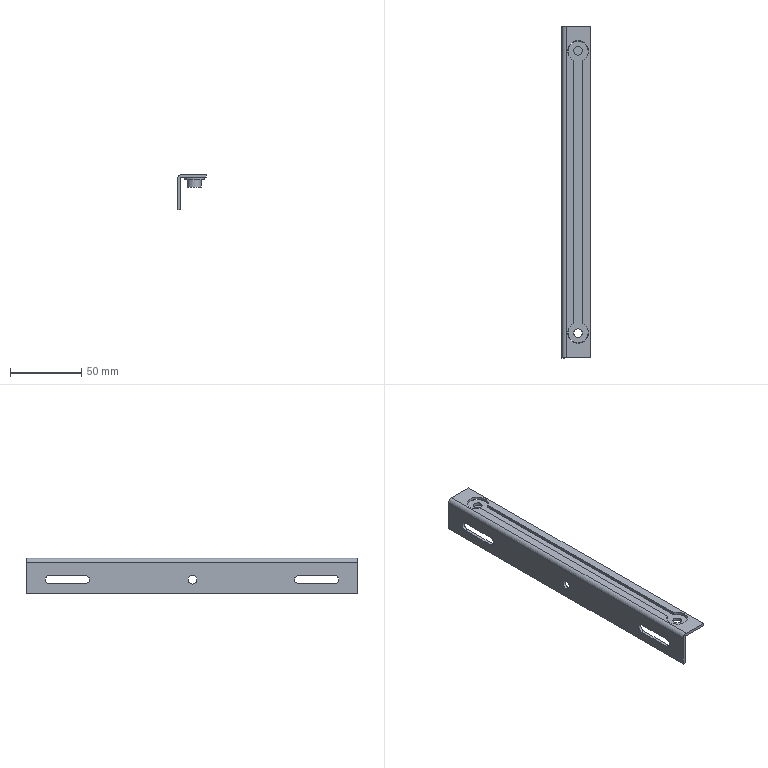Part | SolidWorks | features ICE 4, Extrusion 1 | 2 solids | 42 faces | box 20 x 233 x 25 mm | volume 22029 mm3 | cylinder 22 | plane 20 | commonest cylinder face diameters 14.5 x6 6 x5 6.2 x4 6.3 x2 9.952 x2 14 x2
STEP:
#1=CARTESIAN_POINT('',(-5.5,17.5,-4.));
#2=VERTEX_POINT('',#1);
#3=CARTESIAN_POINT('',(-11.5,17.5,-4.));
#4=VERTEX_POINT('',#3);
#5=CARTESIAN_POINT('',(-8.5,17.5,-4.));
#6=DIRECTION('',(0.,0.,-1.));
#7=DIRECTION('',(-1.,0.,0.));
#8=AXIS2_PLACEMENT_3D('',#5,#6,#7);
#9=CIRCLE('',#8,3.);
#10=EDGE_CURVE('',#2,#4,#9,.T.);
#11=ORIENTED_EDGE('',*,*,#10,.T.);
#12=CARTESIAN_POINT('',(-11.5,17.5,-2.));
#13=VERTEX_POINT('',#12);
#14=CARTESIAN_POINT('',(-11.5,17.5,-4.));
#15=DIRECTION('',(0.,0.,1.));
#16=VECTOR('',#15,1000.);
#17=LINE('',#14,#16);
#18=EDGE_CURVE('',#4,#13,#17,.T.);
#19=ORIENTED_EDGE('',*,*,#18,.T.);
#20=CARTESIAN_POINT('',(-5.5,17.5,-2.));
#21=VERTEX_POINT('',#20);
#22=CARTESIAN_POINT('',(-8.5,17.5,-2.));
#23=DIRECTION('',(0.,0.,-1.));
#24=DIRECTION('',(-1.,0.,0.));
#25=AXIS2_PLACEMENT_3D('',#22,#23,#24);
#26=CIRCLE('',#25,3.);
#27=EDGE_CURVE('',#21,#13,#26,.T.);
#28=ORIENTED_EDGE('',*,*,#27,.F.);
#29=CARTESIAN_POINT('',(-5.5,17.5,-4.));
#30=DIRECTION('',(0.,0.,1.));
#31=VECTOR('',#30,1000.);
#32=LINE('',#29,#31);
#33=EDGE_CURVE('',#2,#21,#32,.T.);
#34=ORIENTED_EDGE('',*,*,#33,.F.);
#35=EDGE_LOOP('',(#11,#19,#28,#34));
#36=FACE_OUTER_BOUND('',#35,.T.);
#37=CARTESIAN_POINT('',(-8.5,17.5,-4.));
#38=DIRECTION('',(0.,0.,1.));
#39=DIRECTION('',(1.,0.,0.));
#40=AXIS2_PLACEMENT_3D('',#37,#38,#39);
#41=CYLINDRICAL_SURFACE('',#40,3.);
#42=ADVANCED_FACE('',(#36),#41,.F.);
#43=CARTESIAN_POINT('',(-5.5,215.5,-4.));
#44=VERTEX_POINT('',#43);
#45=CARTESIAN_POINT('',(-11.5,215.5,-4.));
#46=VERTEX_POINT('',#45);
#47=CARTESIAN_POINT('',(-8.5,215.5,-4.));
#48=DIRECTION('',(0.,0.,-1.));
#49=DIRECTION('',(-1.,0.,0.));
#50=AXIS2_PLACEMENT_3D('',#47,#48,#49);
#51=CIRCLE('',#50,3.);
#52=EDGE_CURVE('',#44,#46,#51,.T.);
#53=ORIENTED_EDGE('',*,*,#52,.T.);
#54=CARTESIAN_POINT('',(-11.5,215.5,-2.));
#55=VERTEX_POINT('',#54);
#56=CARTESIAN_POINT('',(-11.5,215.5,-4.));
#57=DIRECTION('',(0.,0.,1.));
#58=VECTOR('',#57,1000.);
#59=LINE('',#56,#58);
#60=EDGE_CURVE('',#46,#55,#59,.T.);
#61=ORIENTED_EDGE('',*,*,#60,.T.);
#62=CARTESIAN_POINT('',(-5.5,215.5,-2.));
#63=VERTEX_POINT('',#62);
#64=CARTESIAN_POINT('',(-8.5,215.5,-2.));
#65=DIRECTION('',(0.,0.,-1.));
#66=DIRECTION('',(-1.,0.,0.));
#67=AXIS2_PLACEMENT_3D('',#64,#65,#66);
#68=CIRCLE('',#67,3.);
#69=EDGE_CURVE('',#63,#55,#68,.T.);
#70=ORIENTED_EDGE('',*,*,#69,.F.);
#71=CARTESIAN_POINT('',(-5.5,215.5,-4.));
#72=DIRECTION('',(0.,0.,1.));
#73=VECTOR('',#72,1000.);
#74=LINE('',#71,#73);
#75=EDGE_CURVE('',#44,#63,#74,.T.);
#76=ORIENTED_EDGE('',*,*,#75,.F.);
#77=EDGE_LOOP('',(#53,#61,#70,#76));
#78=FACE_OUTER_BOUND('',#77,.T.);
#79=CARTESIAN_POINT('',(-8.5,215.5,-4.));
#80=DIRECTION('',(0.,0.,1.));
#81=DIRECTION('',(1.,0.,0.));
#82=AXIS2_PLACEMENT_3D('',#79,#80,#81);
#83=CYLINDRICAL_SURFACE('',#82,3.);
#84=ADVANCED_FACE('',(#78),#83,.F.);
#85=CARTESIAN_POINT('',(-1.25,215.5,0.));
#86=VERTEX_POINT('',#85);
#87=CARTESIAN_POINT('',(-5.4,208.946,0.));
#88=VERTEX_POINT('',#87);
#89=CARTESIAN_POINT('',(-8.5,215.5,0.));
#90=DIRECTION('',(0.,0.,-1.));
#91=DIRECTION('',(-1.,0.,0.));
#92=AXIS2_PLACEMENT_3D('',#89,#90,#91);
#93=CIRCLE('',#92,7.25);
#94=EDGE_CURVE('',#86,#88,#93,.T.);
#95=ORIENTED_EDGE('',*,*,#94,.F.);
#96=CARTESIAN_POINT('',(-1.25,215.5,-2.));
#97=VERTEX_POINT('',#96);
#98=CARTESIAN_POINT('',(-1.25,215.5,0.));
#99=DIRECTION('',(0.,0.,-1.));
#100=VECTOR('',#99,1000.);
#101=LINE('',#98,#100);
#102=EDGE_CURVE('',#86,#97,#101,.T.);
#103=ORIENTED_EDGE('',*,*,#102,.T.);
#104=CARTESIAN_POINT('',(-1.5,213.613,-2.));
#105=VERTEX_POINT('',#104);
#106=CARTESIAN_POINT('',(-8.5,215.5,-2.));
#107=DIRECTION('',(0.,0.,-1.));
#108=DIRECTION('',(-1.,0.,0.));
#109=AXIS2_PLACEMENT_3D('',#106,#107,#108);
#110=CIRCLE('',#109,7.25);
#111=EDGE_CURVE('',#97,#105,#110,.T.);
#112=ORIENTED_EDGE('',*,*,#111,.T.);
#113=CARTESIAN_POINT('',(-5.4,208.946,-2.));
#114=VERTEX_POINT('',#113);
#115=CARTESIAN_POINT('',(-8.5,215.5,-2.));
#116=DIRECTION('',(0.,0.,1.));
#117=DIRECTION('',(-1.,0.,0.));
#118=AXIS2_PLACEMENT_3D('',#115,#116,#117);
#119=CIRCLE('',#118,7.25);
#120=EDGE_CURVE('',#114,#105,#119,.T.);
#121=ORIENTED_EDGE('',*,*,#120,.F.);
#122=CARTESIAN_POINT('',(-5.4,208.946,0.));
#123=DIRECTION('',(0.,0.,-1.));
#124=VECTOR('',#123,1000.);
#125=LINE('',#122,#124);
#126=EDGE_CURVE('',#88,#114,#125,.T.);
#127=ORIENTED_EDGE('',*,*,#126,.F.);
#128=EDGE_LOOP('',(#95,#103,#112,#121,#127));
#129=FACE_OUTER_BOUND('',#128,.T.);
#130=CARTESIAN_POINT('',(-8.5,215.5,0.));
#131=DIRECTION('',(0.,0.,-1.));
#132=DIRECTION('',(-1.,0.,0.));
#133=AXIS2_PLACEMENT_3D('',#130,#131,#132);
#134=CYLINDRICAL_SURFACE('',#133,7.25);
#135=ADVANCED_FACE('',(#129),#134,.F.);
#136=ORIENTED_EDGE('',*,*,#102,.F.);
#137=CARTESIAN_POINT('',(-15.75,215.5,0.));
#138=VERTEX_POINT('',#137);
#139=CARTESIAN_POINT('',(-8.5,215.5,0.));
#140=DIRECTION('',(0.,0.,-1.));
#141=DIRECTION('',(-1.,0.,0.));
#142=AXIS2_PLACEMENT_3D('',#139,#140,#141);
#143=CIRCLE('',#142,7.25);
#144=EDGE_CURVE('',#138,#86,#143,.T.);
#145=ORIENTED_EDGE('',*,*,#144,.F.);
#146=CARTESIAN_POINT('',(-15.75,215.5,-2.));
#147=VERTEX_POINT('',#146);
#148=CARTESIAN_POINT('',(-15.75,215.5,0.));
#149=DIRECTION('',(0.,0.,-1.));
#150=VECTOR('',#149,1000.);
#151=LINE('',#148,#150);
#152=EDGE_CURVE('',#138,#147,#151,.T.);
#153=ORIENTED_EDGE('',*,*,#152,.T.);
#154=CARTESIAN_POINT('',(-8.5,215.5,-2.));
#155=DIRECTION('',(0.,0.,-1.));
#156=DIRECTION('',(-1.,0.,0.));
#157=AXIS2_PLACEMENT_3D('',#154,#155,#156);
#158=CIRCLE('',#157,7.25);
#159=EDGE_CURVE('',#147,#97,#158,.T.);
#160=ORIENTED_EDGE('',*,*,#159,.T.);
#161=EDGE_LOOP('',(#136,#145,#153,#160));
#162=FACE_OUTER_BOUND('',#161,.T.);
#163=CARTESIAN_POINT('',(-8.5,215.5,0.));
#164=DIRECTION('',(0.,0.,-1.));
#165=DIRECTION('',(-1.,0.,0.));
#166=AXIS2_PLACEMENT_3D('',#163,#164,#165);
#167=CYLINDRICAL_SURFACE('',#166,7.25);
#168=ADVANCED_FACE('',(#162),#167,.F.);
#169=CARTESIAN_POINT('',(-1.25,17.5,0.));
#170=VERTEX_POINT('',#169);
#171=CARTESIAN_POINT('',(-15.75,17.5,0.));
#172=VERTEX_POINT('',#171);
#173=CARTESIAN_POINT('',(-8.5,17.5,0.));
#174=DIRECTION('',(0.,0.,-1.));
#175=DIRECTION('',(-1.,0.,0.));
#176=AXIS2_PLACEMENT_3D('',#173,#174,#175);
#177=CIRCLE('',#176,7.25);
#178=EDGE_CURVE('',#170,#172,#177,.T.);
#179=ORIENTED_EDGE('',*,*,#178,.F.);
#180=CARTESIAN_POINT('',(-1.25,17.5,-2.));
#181=VERTEX_POINT('',#180);
#182=CARTESIAN_POINT('',(-1.25,17.5,0.));
#183=DIRECTION('',(0.,0.,-1.));
#184=VECTOR('',#183,1000.);
#185=LINE('',#182,#184);
#186=EDGE_CURVE('',#170,#181,#185,.T.);
#187=ORIENTED_EDGE('',*,*,#186,.T.);
#188=CARTESIAN_POINT('',(-15.75,17.5,-2.));
#189=VERTEX_POINT('',#188);
#190=CARTESIAN_POINT('',(-8.5,17.5,-2.));
#191=DIRECTION('',(0.,0.,-1.));
#192=DIRECTION('',(-1.,0.,0.));
#193=AXIS2_PLACEMENT_3D('',#190,#191,#192);
#194=CIRCLE('',#193,7.25);
#195=EDGE_CURVE('',#181,#189,#194,.T.);
#196=ORIENTED_EDGE('',*,*,#195,.T.);
#197=CARTESIAN_POINT('',(-15.75,17.5,0.));
#198=DIRECTION('',(0.,0.,-1.));
#199=VECTOR('',#198,1000.);
#200=LINE('',#197,#199);
#201=EDGE_CURVE('',#172,#189,#200,.T.);
#202=ORIENTED_EDGE('',*,*,#201,.F.);
#203=EDGE_LOOP('',(#179,#187,#196,#202));
#204=FACE_OUTER_BOUND('',#203,.T.);
#205=CARTESIAN_POINT('',(-8.5,17.5,0.));
#206=DIRECTION('',(0.,0.,-1.));
#207=DIRECTION('',(-1.,0.,0.));
#208=AXIS2_PLACEMENT_3D('',#205,#206,#207);
#209=CYLINDRICAL_SURFACE('',#208,7.25);
#210=ADVANCED_FACE('',(#204),#209,.F.);
#211=CARTESIAN_POINT('',(-11.6,24.054,0.));
#212=VERTEX_POINT('',#211);
#213=CARTESIAN_POINT('',(-8.5,17.5,0.));
#214=DIRECTION('',(0.,0.,-1.));
#215=DIRECTION('',(-1.,0.,0.));
#216=AXIS2_PLACEMENT_3D('',#213,#214,#215);
#217=CIRCLE('',#216,7.25);
#218=EDGE_CURVE('',#172,#212,#217,.T.);
#219=ORIENTED_EDGE('',*,*,#218,.F.);
#220=ORIENTED_EDGE('',*,*,#201,.T.);
#221=CARTESIAN_POINT('',(-15.5,19.387,-2.));
#222=VERTEX_POINT('',#221);
#223=CARTESIAN_POINT('',(-8.5,17.5,-2.));
#224=DIRECTION('',(0.,0.,-1.));
#225=DIRECTION('',(-1.,0.,0.));
#226=AXIS2_PLACEMENT_3D('',#223,#224,#225);
#227=CIRCLE('',#226,7.25);
#228=EDGE_CURVE('',#189,#222,#227,.T.);
#229=ORIENTED_EDGE('',*,*,#228,.T.);
#230=CARTESIAN_POINT('',(-11.6,24.054,-2.));
#231=VERTEX_POINT('',#230);
#232=CARTESIAN_POINT('',(-8.5,17.5,-2.));
#233=DIRECTION('',(0.,0.,1.));
#234=DIRECTION('',(-1.,0.,0.));
#235=AXIS2_PLACEMENT_3D('',#232,#233,#234);
#236=CIRCLE('',#235,7.25);
#237=EDGE_CURVE('',#231,#222,#236,.T.);
#238=ORIENTED_EDGE('',*,*,#237,.F.);
#239=CARTESIAN_POINT('',(-11.6,24.054,0.));
#240=DIRECTION('',(0.,0.,-1.));
#241=VECTOR('',#240,1000.);
#242=LINE('',#239,#241);
#243=EDGE_CURVE('',#212,#231,#242,.T.);
#244=ORIENTED_EDGE('',*,*,#243,.F.);
#245=EDGE_LOOP('',(#219,#220,#229,#238,#244));
#246=FACE_OUTER_BOUND('',#245,.T.);
#247=CARTESIAN_POINT('',(-8.5,17.5,0.));
#248=DIRECTION('',(0.,0.,-1.));
#249=DIRECTION('',(-1.,0.,0.));
#250=AXIS2_PLACEMENT_3D('',#247,#248,#249);
#251=CYLINDRICAL_SURFACE('',#250,7.25);
#252=ADVANCED_FACE('',(#246),#251,.F.);
#253=CARTESIAN_POINT('',(-20.,116.173,-11.85));
#254=VERTEX_POINT('',#253);
#255=CARTESIAN_POINT('',(-20.,116.173,-18.15));
#256=VERTEX_POINT('',#255);
#257=CARTESIAN_POINT('',(-20.,116.173,-15.));
#258=DIRECTION('',(1.,0.,0.));
#259=DIRECTION('',(0.,0.,-1.));
#260=AXIS2_PLACEMENT_3D('',#257,#258,#259);
#261=CIRCLE('',#260,3.15);
#262=EDGE_CURVE('',#254,#256,#261,.T.);
#263=ORIENTED_EDGE('',*,*,#262,.F.);
#264=CARTESIAN_POINT('',(-18.,116.173,-11.85));
#265=VERTEX_POINT('',#264);
#266=CARTESIAN_POINT('',(-20.,116.173,-11.85));
#267=DIRECTION('',(1.,0.,0.));
#268=VECTOR('',#267,1000.);
#269=LINE('',#266,#268);
#270=EDGE_CURVE('',#254,#265,#269,.T.);
#271=ORIENTED_EDGE('',*,*,#270,.T.);
#272=CARTESIAN_POINT('',(-18.,116.173,-18.15));
#273=VERTEX_POINT('',#272);
#274=CARTESIAN_POINT('',(-18.,116.173,-15.));
#275=DIRECTION('',(-1.,0.,0.));
#276=DIRECTION('',(0.,0.,1.));
#277=AXIS2_PLACEMENT_3D('',#274,#275,#276);
#278=CIRCLE('',#277,3.15);
#279=EDGE_CURVE('',#273,#265,#278,.T.);
#280=ORIENTED_EDGE('',*,*,#279,.F.);
#281=CARTESIAN_POINT('',(-20.,116.173,-18.15));
#282=DIRECTION('',(1.,0.,0.));
#283=VECTOR('',#282,1000.);
#284=LINE('',#281,#283);
#285=EDGE_CURVE('',#256,#273,#284,.T.);
#286=ORIENTED_EDGE('',*,*,#285,.F.);
#287=EDGE_LOOP('',(#263,#271,#280,#286));
#288=FACE_OUTER_BOUND('',#287,.T.);
#289=CARTESIAN_POINT('',(-20.,116.173,-15.));
#290=DIRECTION('',(1.,0.,0.));
#291=DIRECTION('',(0.,0.,-1.));
#292=AXIS2_PLACEMENT_3D('',#289,#290,#291);
#293=CYLINDRICAL_SURFACE('',#292,3.15);
#294=ADVANCED_FACE('',(#288),#293,.F.);
#295=CARTESIAN_POINT('',(0.,0.,-2.));
#296=VERTEX_POINT('',#295);
#297=CARTESIAN_POINT('',(-17.,0.,-2.));
#298=VERTEX_POINT('',#297);
#299=CARTESIAN_POINT('',(0.,0.,-2.));
#300=DIRECTION('',(-1.,0.,0.));
#301=VECTOR('',#300,1000.);
#302=LINE('',#299,#301);
#303=EDGE_CURVE('',#296,#298,#302,.T.);
#304=ORIENTED_EDGE('',*,*,#303,.T.);
#305=CARTESIAN_POINT('',(-17.,233.,-2.));
#306=VERTEX_POINT('',#305);
#307=CARTESIAN_POINT('',(-17.,233.,-2.));
#308=DIRECTION('',(0.,-1.,0.));
#309=VECTOR('',#308,1000.);
#310=LINE('',#307,#309);
#311=EDGE_CURVE('',#306,#298,#310,.T.);
#312=ORIENTED_EDGE('',*,*,#311,.F.);
#313=CARTESIAN_POINT('',(0.,233.,-2.));
#314=VERTEX_POINT('',#313);
#315=CARTESIAN_POINT('',(0.,233.,-2.));
#316=DIRECTION('',(-1.,0.,0.));
#317=VECTOR('',#316,1000.);
#318=LINE('',#315,#317);
#319=EDGE_CURVE('',#314,#306,#318,.T.);
#320=ORIENTED_EDGE('',*,*,#319,.F.);
#321=CARTESIAN_POINT('',(0.,233.,-2.));
#322=DIRECTION('',(0.,-1.,0.));
#323=VECTOR('',#322,1000.);
#324=LINE('',#321,#323);
#325=EDGE_CURVE('',#314,#296,#324,.T.);
#326=ORIENTED_EDGE('',*,*,#325,.T.);
#327=EDGE_LOOP('',(#304,#312,#320,#326));
#328=FACE_OUTER_BOUND('',#327,.T.);
#329=CARTESIAN_POINT('',(-15.5,213.613,-2.));
#330=VERTEX_POINT('',#329);
#331=CARTESIAN_POINT('',(-15.5,215.5,-2.));
#332=DIRECTION('',(0.,1.,0.));
#333=VECTOR('',#332,1000.);
#334=LINE('',#331,#333);
#335=EDGE_CURVE('',#222,#330,#334,.T.);
#336=ORIENTED_EDGE('',*,*,#335,.F.);
#337=ORIENTED_EDGE('',*,*,#228,.F.);
#338=ORIENTED_EDGE('',*,*,#195,.F.);
#339=CARTESIAN_POINT('',(-1.5,19.387,-2.));
#340=VERTEX_POINT('',#339);
#341=CARTESIAN_POINT('',(-8.5,17.5,-2.));
#342=DIRECTION('',(0.,0.,-1.));
#343=DIRECTION('',(-1.,0.,0.));
#344=AXIS2_PLACEMENT_3D('',#341,#342,#343);
#345=CIRCLE('',#344,7.25);
#346=EDGE_CURVE('',#340,#181,#345,.T.);
#347=ORIENTED_EDGE('',*,*,#346,.F.);
#348=CARTESIAN_POINT('',(-1.5,215.5,-2.));
#349=DIRECTION('',(0.,-1.,0.));
#350=VECTOR('',#349,1000.);
#351=LINE('',#348,#350);
#352=EDGE_CURVE('',#105,#340,#351,.T.);
#353=ORIENTED_EDGE('',*,*,#352,.F.);
#354=ORIENTED_EDGE('',*,*,#111,.F.);
#355=ORIENTED_EDGE('',*,*,#159,.F.);
#356=CARTESIAN_POINT('',(-8.5,215.5,-2.));
#357=DIRECTION('',(0.,0.,-1.));
#358=DIRECTION('',(-1.,0.,0.));
#359=AXIS2_PLACEMENT_3D('',#356,#357,#358);
#360=CIRCLE('',#359,7.25);
#361=EDGE_CURVE('',#330,#147,#360,.T.);
#362=ORIENTED_EDGE('',*,*,#361,.F.);
#363=EDGE_LOOP('',(#336,#337,#338,#347,#353,#354,#355,#362));
#364=FACE_BOUND('',#363,.T.);
#365=CARTESIAN_POINT('',(0.,233.,-2.));
#366=DIRECTION('',(0.,0.,1.));
#367=DIRECTION('',(1.,0.,0.));
#368=AXIS2_PLACEMENT_3D('',#365,#366,#367);
#369=PLANE('',#368);
#370=ADVANCED_FACE('',(#328,#364),#369,.F.);
#371=CARTESIAN_POINT('',(0.,0.,0.));
#372=VERTEX_POINT('',#371);
#373=CARTESIAN_POINT('',(0.,0.,-2.));
#374=DIRECTION('',(0.,0.,-1.));
#375=VECTOR('',#374,1000.);
#376=LINE('',#373,#375);
#377=EDGE_CURVE('',#372,#296,#376,.T.);
#378=ORIENTED_EDGE('',*,*,#377,.T.);
#379=ORIENTED_EDGE('',*,*,#325,.F.);
#380=CARTESIAN_POINT('',(0.,233.,0.));
#381=VERTEX_POINT('',#380);
#382=CARTESIAN_POINT('',(0.,233.,-2.));
#383=DIRECTION('',(0.,0.,-1.));
#384=VECTOR('',#383,1000.);
#385=LINE('',#382,#384);
#386=EDGE_CURVE('',#381,#314,#385,.T.);
#387=ORIENTED_EDGE('',*,*,#386,.F.);
#388=CARTESIAN_POINT('',(0.,233.,0.));
#389=DIRECTION('',(0.,-1.,0.));
#390=VECTOR('',#389,1000.);
#391=LINE('',#388,#390);
#392=EDGE_CURVE('',#381,#372,#391,.T.);
#393=ORIENTED_EDGE('',*,*,#392,.T.);
#394=EDGE_LOOP('',(#378,#379,#387,#393));
#395=FACE_OUTER_BOUND('',#394,.T.);
#396=CARTESIAN_POINT('',(0.,233.,-2.));
#397=DIRECTION('',(-1.,0.,0.));
#398=DIRECTION('',(0.,0.,1.));
#399=AXIS2_PLACEMENT_3D('',#396,#397,#398);
#400=PLANE('',#399);
#401=ADVANCED_FACE('',(#395),#400,.F.);
#402=CARTESIAN_POINT('',(-18.,0.,-3.));
#403=VERTEX_POINT('',#402);
#404=CARTESIAN_POINT('',(-17.,0.,-3.));
#405=DIRECTION('',(0.,-1.,0.));
#406=DIRECTION('',(0.,0.,-1.));
#407=AXIS2_PLACEMENT_3D('',#404,#405,#406);
#408=CIRCLE('',#407,1.);
#409=EDGE_CURVE('',#298,#403,#408,.T.);
#410=ORIENTED_EDGE('',*,*,#409,.T.);
#411=CARTESIAN_POINT('',(-18.,233.,-3.));
#412=VERTEX_POINT('',#411);
#413=CARTESIAN_POINT('',(-18.,233.,-3.));
#414=DIRECTION('',(0.,-1.,0.));
#415=VECTOR('',#414,1000.);
#416=LINE('',#413,#415);
#417=EDGE_CURVE('',#412,#403,#416,.T.);
#418=ORIENTED_EDGE('',*,*,#417,.F.);
#419=CARTESIAN_POINT('',(-17.,233.,-3.));
#420=DIRECTION('',(0.,-1.,0.));
#421=DIRECTION('',(0.,0.,-1.));
#422=AXIS2_PLACEMENT_3D('',#419,#420,#421);
#423=CIRCLE('',#422,1.);
#424=EDGE_CURVE('',#306,#412,#423,.T.);
#425=ORIENTED_EDGE('',*,*,#424,.F.);
#426=ORIENTED_EDGE('',*,*,#311,.T.);
#427=EDGE_LOOP('',(#410,#418,#425,#426));
#428=FACE_OUTER_BOUND('',#427,.T.);
#429=CARTESIAN_POINT('',(-17.,233.,-3.));
#430=DIRECTION('',(0.,-1.,0.));
#431=DIRECTION('',(0.,0.,-1.));
#432=AXIS2_PLACEMENT_3D('',#429,#430,#431);
#433=CYLINDRICAL_SURFACE('',#432,1.);
#434=ADVANCED_FACE('',(#428),#433,.F.);
#435=CARTESIAN_POINT('',(-18.,191.65,-11.9));
#436=VERTEX_POINT('',#435);
#437=CARTESIAN_POINT('',(-18.,216.35,-11.9));
#438=VERTEX_POINT('',#437);
#439=CARTESIAN_POINT('',(-18.,233.,-11.9));
#440=DIRECTION('',(0.,1.,0.));
#441=VECTOR('',#440,1000.);
#442=LINE('',#439,#441);
#443=EDGE_CURVE('',#436,#438,#442,.T.);
#444=ORIENTED_EDGE('',*,*,#443,.T.);
#445=CARTESIAN_POINT('',(-18.,216.35,-18.1));
#446=VERTEX_POINT('',#445);
#447=CARTESIAN_POINT('',(-18.,216.35,-15.));
#448=DIRECTION('',(-1.,0.,0.));
#449=DIRECTION('',(0.,0.,1.));
#450=AXIS2_PLACEMENT_3D('',#447,#448,#449);
#451=CIRCLE('',#450,3.1);
#452=EDGE_CURVE('',#438,#446,#451,.T.);
#453=ORIENTED_EDGE('',*,*,#452,.T.);
#454=CARTESIAN_POINT('',(-18.,191.65,-18.1));
#455=VERTEX_POINT('',#454);
#456=CARTESIAN_POINT('',(-18.,233.,-18.1));
#457=DIRECTION('',(0.,-1.,0.));
#458=VECTOR('',#457,1000.);
#459=LINE('',#456,#458);
#460=EDGE_CURVE('',#446,#455,#459,.T.);
#461=ORIENTED_EDGE('',*,*,#460,.T.);
#462=CARTESIAN_POINT('',(-18.,191.65,-15.));
#463=DIRECTION('',(-1.,0.,0.));
#464=DIRECTION('',(0.,0.,1.));
#465=AXIS2_PLACEMENT_3D('',#462,#463,#464);
#466=CIRCLE('',#465,3.1);
#467=EDGE_CURVE('',#455,#436,#466,.T.);
#468=ORIENTED_EDGE('',*,*,#467,.T.);
#469=EDGE_LOOP('',(#444,#453,#461,#468));
#470=FACE_BOUND('',#469,.T.);
#471=CARTESIAN_POINT('',(-18.,16.65,-11.9));
#472=VERTEX_POINT('',#471);
#473=CARTESIAN_POINT('',(-18.,41.35,-11.9));
#474=VERTEX_POINT('',#473);
#475=CARTESIAN_POINT('',(-18.,233.,-11.9));
#476=DIRECTION('',(0.,1.,0.));
#477=VECTOR('',#476,1000.);
#478=LINE('',#475,#477);
#479=EDGE_CURVE('',#472,#474,#478,.T.);
#480=ORIENTED_EDGE('',*,*,#479,.T.);
#481=CARTESIAN_POINT('',(-18.,41.35,-18.1));
#482=VERTEX_POINT('',#481);
#483=CARTESIAN_POINT('',(-18.,41.35,-15.));
#484=DIRECTION('',(-1.,0.,0.));
#485=DIRECTION('',(0.,0.,1.));
#486=AXIS2_PLACEMENT_3D('',#483,#484,#485);
#487=CIRCLE('',#486,3.1);
#488=EDGE_CURVE('',#474,#482,#487,.T.);
#489=ORIENTED_EDGE('',*,*,#488,.T.);
#490=CARTESIAN_POINT('',(-18.,16.65,-18.1));
#491=VERTEX_POINT('',#490);
#492=CARTESIAN_POINT('',(-18.,233.,-18.1));
#493=DIRECTION('',(0.,-1.,0.));
#494=VECTOR('',#493,1000.);
#495=LINE('',#492,#494);
#496=EDGE_CURVE('',#482,#491,#495,.T.);
#497=ORIENTED_EDGE('',*,*,#496,.T.);
#498=CARTESIAN_POINT('',(-18.,16.65,-15.));
#499=DIRECTION('',(-1.,0.,0.));
#500=DIRECTION('',(0.,0.,1.));
#501=AXIS2_PLACEMENT_3D('',#498,#499,#500);
#502=CIRCLE('',#501,3.1);
#503=EDGE_CURVE('',#491,#472,#502,.T.);
#504=ORIENTED_EDGE('',*,*,#503,.T.);
#505=EDGE_LOOP('',(#480,#489,#497,#504));
#506=FACE_BOUND('',#505,.T.);
#507=ORIENTED_EDGE('',*,*,#279,.T.);
#508=CARTESIAN_POINT('',(-18.,116.173,-15.));
#509=DIRECTION('',(-1.,0.,0.));
#510=DIRECTION('',(0.,0.,1.));
#511=AXIS2_PLACEMENT_3D('',#508,#509,#510);
#512=CIRCLE('',#511,3.15);
#513=EDGE_CURVE('',#265,#273,#512,.T.);
#514=ORIENTED_EDGE('',*,*,#513,.T.);
#515=EDGE_LOOP('',(#507,#514));
#516=FACE_BOUND('',#515,.T.);
#517=CARTESIAN_POINT('',(-18.,0.,-25.));
#518=VERTEX_POINT('',#517);
#519=CARTESIAN_POINT('',(-18.,0.,-25.));
#520=DIRECTION('',(0.,0.,-1.));
#521=VECTOR('',#520,1000.);
#522=LINE('',#519,#521);
#523=EDGE_CURVE('',#403,#518,#522,.T.);
#524=ORIENTED_EDGE('',*,*,#523,.T.);
#525=CARTESIAN_POINT('',(-18.,233.,-25.));
#526=VERTEX_POINT('',#525);
#527=CARTESIAN_POINT('',(-18.,233.,-25.));
#528=DIRECTION('',(0.,-1.,0.));
#529=VECTOR('',#528,1000.);
#530=LINE('',#527,#529);
#531=EDGE_CURVE('',#526,#518,#530,.T.);
#532=ORIENTED_EDGE('',*,*,#531,.F.);
#533=CARTESIAN_POINT('',(-18.,233.,-3.));
#534=DIRECTION('',(0.,0.,-1.));
#535=VECTOR('',#534,1000.);
#536=LINE('',#533,#535);
#537=EDGE_CURVE('',#412,#526,#536,.T.);
#538=ORIENTED_EDGE('',*,*,#537,.F.);
#539=ORIENTED_EDGE('',*,*,#417,.T.);
#540=EDGE_LOOP('',(#524,#532,#538,#539));
#541=FACE_OUTER_BOUND('',#540,.T.);
#542=CARTESIAN_POINT('',(-18.,233.,-25.));
#543=DIRECTION('',(-1.,0.,0.));
#544=DIRECTION('',(0.,0.,1.));
#545=AXIS2_PLACEMENT_3D('',#542,#543,#544);
#546=PLANE('',#545);
#547=ADVANCED_FACE('',(#470,#506,#516,#541),#546,.F.);
#548=CARTESIAN_POINT('',(-20.,0.,-25.));
#549=VERTEX_POINT('',#548);
#550=CARTESIAN_POINT('',(-20.,0.,-25.));
#551=DIRECTION('',(-1.,0.,0.));
#552=VECTOR('',#551,1000.);
#553=LINE('',#550,#552);
#554=EDGE_CURVE('',#518,#549,#553,.T.);
#555=ORIENTED_EDGE('',*,*,#554,.T.);
#556=CARTESIAN_POINT('',(-20.,233.,-25.));
#557=VERTEX_POINT('',#556);
#558=CARTESIAN_POINT('',(-20.,233.,-25.));
#559=DIRECTION('',(0.,-1.,0.));
#560=VECTOR('',#559,1000.);
#561=LINE('',#558,#560);
#562=EDGE_CURVE('',#557,#549,#561,.T.);
#563=ORIENTED_EDGE('',*,*,#562,.F.);
#564=CARTESIAN_POINT('',(-20.,233.,-25.));
#565=DIRECTION('',(-1.,0.,0.));
#566=VECTOR('',#565,1000.);
#567=LINE('',#564,#566);
#568=EDGE_CURVE('',#526,#557,#567,.T.);
#569=ORIENTED_EDGE('',*,*,#568,.F.);
#570=ORIENTED_EDGE('',*,*,#531,.T.);
#571=EDGE_LOOP('',(#555,#563,#569,#570));
#572=FACE_OUTER_BOUND('',#571,.T.);
#573=CARTESIAN_POINT('',(-20.,233.,-25.));
#574=DIRECTION('',(0.,0.,1.));
#575=DIRECTION('',(1.,0.,0.));
#576=AXIS2_PLACEMENT_3D('',#573,#574,#575);
#577=PLANE('',#576);
#578=ADVANCED_FACE('',(#572),#577,.F.);
#579=CARTESIAN_POINT('',(-20.,191.65,-18.1));
#580=VERTEX_POINT('',#579);
#581=CARTESIAN_POINT('',(-20.,216.35,-18.1));
#582=VERTEX_POINT('',#581);
#583=CARTESIAN_POINT('',(-20.,216.35,-18.1));
#584=DIRECTION('',(0.,1.,0.));
#585=VECTOR('',#584,1000.);
#586=LINE('',#583,#585);
#587=EDGE_CURVE('',#580,#582,#586,.T.);
#588=ORIENTED_EDGE('',*,*,#587,.T.);
#589=CARTESIAN_POINT('',(-20.,216.35,-11.9));
#590=VERTEX_POINT('',#589);
#591=CARTESIAN_POINT('',(-20.,216.35,-15.));
#592=DIRECTION('',(1.,0.,0.));
#593=DIRECTION('',(0.,0.,-1.));
#594=AXIS2_PLACEMENT_3D('',#591,#592,#593);
#595=CIRCLE('',#594,3.1);
#596=EDGE_CURVE('',#582,#590,#595,.T.);
#597=ORIENTED_EDGE('',*,*,#596,.T.);
#598=CARTESIAN_POINT('',(-20.,191.65,-11.9));
#599=VERTEX_POINT('',#598);
#600=CARTESIAN_POINT('',(-20.,216.35,-11.9));
#601=DIRECTION('',(0.,-1.,0.));
#602=VECTOR('',#601,1000.);
#603=LINE('',#600,#602);
#604=EDGE_CURVE('',#590,#599,#603,.T.);
#605=ORIENTED_EDGE('',*,*,#604,.T.);
#606=CARTESIAN_POINT('',(-20.,191.65,-15.));
#607=DIRECTION('',(1.,0.,0.));
#608=DIRECTION('',(0.,0.,-1.));
#609=AXIS2_PLACEMENT_3D('',#606,#607,#608);
#610=CIRCLE('',#609,3.1);
#611=EDGE_CURVE('',#599,#580,#610,.T.);
#612=ORIENTED_EDGE('',*,*,#611,.T.);
#613=EDGE_LOOP('',(#588,#597,#605,#612));
#614=FACE_BOUND('',#613,.T.);
#615=CARTESIAN_POINT('',(-20.,16.65,-18.1));
#616=VERTEX_POINT('',#615);
#617=CARTESIAN_POINT('',(-20.,41.35,-18.1));
#618=VERTEX_POINT('',#617);
#619=CARTESIAN_POINT('',(-20.,41.35,-18.1));
#620=DIRECTION('',(0.,1.,0.));
#621=VECTOR('',#620,1000.);
#622=LINE('',#619,#621);
#623=EDGE_CURVE('',#616,#618,#622,.T.);
#624=ORIENTED_EDGE('',*,*,#623,.T.);
#625=CARTESIAN_POINT('',(-20.,41.35,-11.9));
#626=VERTEX_POINT('',#625);
#627=CARTESIAN_POINT('',(-20.,41.35,-15.));
#628=DIRECTION('',(1.,0.,0.));
#629=DIRECTION('',(0.,0.,-1.));
#630=AXIS2_PLACEMENT_3D('',#627,#628,#629);
#631=CIRCLE('',#630,3.1);
#632=EDGE_CURVE('',#618,#626,#631,.T.);
#633=ORIENTED_EDGE('',*,*,#632,.T.);
#634=CARTESIAN_POINT('',(-20.,16.65,-11.9));
#635=VERTEX_POINT('',#634);
#636=CARTESIAN_POINT('',(-20.,41.35,-11.9));
#637=DIRECTION('',(0.,-1.,0.));
#638=VECTOR('',#637,1000.);
#639=LINE('',#636,#638);
#640=EDGE_CURVE('',#626,#635,#639,.T.);
#641=ORIENTED_EDGE('',*,*,#640,.T.);
#642=CARTESIAN_POINT('',(-20.,16.65,-15.));
#643=DIRECTION('',(1.,0.,0.));
#644=DIRECTION('',(0.,0.,-1.));
#645=AXIS2_PLACEMENT_3D('',#642,#643,#644);
#646=CIRCLE('',#645,3.1);
#647=EDGE_CURVE('',#635,#616,#646,.T.);
#648=ORIENTED_EDGE('',*,*,#647,.T.);
#649=EDGE_LOOP('',(#624,#633,#641,#648));
#650=FACE_BOUND('',#649,.T.);
#651=CARTESIAN_POINT('',(-20.,116.173,-15.));
#652=DIRECTION('',(1.,0.,0.));
#653=DIRECTION('',(0.,0.,-1.));
#654=AXIS2_PLACEMENT_3D('',#651,#652,#653);
#655=CIRCLE('',#654,3.15);
#656=EDGE_CURVE('',#256,#254,#655,.T.);
#657=ORIENTED_EDGE('',*,*,#656,.T.);
#658=ORIENTED_EDGE('',*,*,#262,.T.);
#659=EDGE_LOOP('',(#657,#658));
#660=FACE_BOUND('',#659,.T.);
#661=CARTESIAN_POINT('',(-20.,0.,-3.));
#662=VERTEX_POINT('',#661);
#663=CARTESIAN_POINT('',(-20.,0.,-3.));
#664=DIRECTION('',(0.,0.,1.));
#665=VECTOR('',#664,1000.);
#666=LINE('',#663,#665);
#667=EDGE_CURVE('',#549,#662,#666,.T.);
#668=ORIENTED_EDGE('',*,*,#667,.T.);
#669=CARTESIAN_POINT('',(-20.,233.,-3.));
#670=VERTEX_POINT('',#669);
#671=CARTESIAN_POINT('',(-20.,233.,-3.));
#672=DIRECTION('',(0.,-1.,0.));
#673=VECTOR('',#672,1000.);
#674=LINE('',#671,#673);
#675=EDGE_CURVE('',#670,#662,#674,.T.);
#676=ORIENTED_EDGE('',*,*,#675,.F.);
#677=CARTESIAN_POINT('',(-20.,233.,-8.424));
#678=DIRECTION('',(0.,0.,1.));
#679=VECTOR('',#678,1000.);
#680=LINE('',#677,#679);
#681=EDGE_CURVE('',#557,#670,#680,.T.);
#682=ORIENTED_EDGE('',*,*,#681,.F.);
#683=ORIENTED_EDGE('',*,*,#562,.T.);
#684=EDGE_LOOP('',(#668,#676,#682,#683));
#685=FACE_OUTER_BOUND('',#684,.T.);
#686=CARTESIAN_POINT('',(-20.,233.,-3.));
#687=DIRECTION('',(1.,0.,0.));
#688=DIRECTION('',(0.,0.,-1.));
#689=AXIS2_PLACEMENT_3D('',#686,#687,#688);
#690=PLANE('',#689);
#691=ADVANCED_FACE('',(#614,#650,#660,#685),#690,.F.);
#692=CARTESIAN_POINT('',(-17.,0.,0.));
#693=VERTEX_POINT('',#692);
#694=CARTESIAN_POINT('',(-17.,0.,-3.));
#695=DIRECTION('',(0.,1.,0.));
#696=DIRECTION('',(0.,0.,-1.));
#697=AXIS2_PLACEMENT_3D('',#694,#695,#696);
#698=CIRCLE('',#697,3.);
#699=EDGE_CURVE('',#662,#693,#698,.T.);
#700=ORIENTED_EDGE('',*,*,#699,.T.);
#701=CARTESIAN_POINT('',(-17.,233.,0.));
#702=VERTEX_POINT('',#701);
#703=CARTESIAN_POINT('',(-17.,233.,0.));
#704=DIRECTION('',(0.,-1.,0.));
#705=VECTOR('',#704,1000.);
#706=LINE('',#703,#705);
#707=EDGE_CURVE('',#702,#693,#706,.T.);
#708=ORIENTED_EDGE('',*,*,#707,.F.);
#709=CARTESIAN_POINT('',(-17.,233.,-3.));
#710=DIRECTION('',(0.,1.,0.));
#711=DIRECTION('',(0.,0.,-1.));
#712=AXIS2_PLACEMENT_3D('',#709,#710,#711);
#713=CIRCLE('',#712,3.);
#714=EDGE_CURVE('',#670,#702,#713,.T.);
#715=ORIENTED_EDGE('',*,*,#714,.F.);
#716=ORIENTED_EDGE('',*,*,#675,.T.);
#717=EDGE_LOOP('',(#700,#708,#715,#716));
#718=FACE_OUTER_BOUND('',#717,.T.);
#719=CARTESIAN_POINT('',(-17.,233.,-3.));
#720=DIRECTION('',(0.,-1.,0.));
#721=DIRECTION('',(0.,0.,-1.));
#722=AXIS2_PLACEMENT_3D('',#719,#720,#721);
#723=CYLINDRICAL_SURFACE('',#722,3.);
#724=ADVANCED_FACE('',(#718),#723,.T.);
#725=CARTESIAN_POINT('',(-5.4,24.054,0.));
#726=VERTEX_POINT('',#725);
#727=CARTESIAN_POINT('',(-5.4,208.946,0.));
#728=DIRECTION('',(0.,-1.,0.));
#729=VECTOR('',#728,1000.);
#730=LINE('',#727,#729);
#731=EDGE_CURVE('',#88,#726,#730,.T.);
#732=ORIENTED_EDGE('',*,*,#731,.T.);
#733=CARTESIAN_POINT('',(-8.5,17.5,0.));
#734=DIRECTION('',(0.,0.,-1.));
#735=DIRECTION('',(-1.,0.,0.));
#736=AXIS2_PLACEMENT_3D('',#733,#734,#735);
#737=CIRCLE('',#736,7.25);
#738=EDGE_CURVE('',#726,#170,#737,.T.);
#739=ORIENTED_EDGE('',*,*,#738,.T.);
#740=ORIENTED_EDGE('',*,*,#178,.T.);
#741=ORIENTED_EDGE('',*,*,#218,.T.);
#742=CARTESIAN_POINT('',(-11.6,208.946,0.));
#743=VERTEX_POINT('',#742);
#744=CARTESIAN_POINT('',(-11.6,208.946,0.));
#745=DIRECTION('',(0.,1.,0.));
#746=VECTOR('',#745,1000.);
#747=LINE('',#744,#746);
#748=EDGE_CURVE('',#212,#743,#747,.T.);
#749=ORIENTED_EDGE('',*,*,#748,.T.);
#750=CARTESIAN_POINT('',(-8.5,215.5,0.));
#751=DIRECTION('',(0.,0.,-1.));
#752=DIRECTION('',(-1.,0.,0.));
#753=AXIS2_PLACEMENT_3D('',#750,#751,#752);
#754=CIRCLE('',#753,7.25);
#755=EDGE_CURVE('',#743,#138,#754,.T.);
#756=ORIENTED_EDGE('',*,*,#755,.T.);
#757=ORIENTED_EDGE('',*,*,#144,.T.);
#758=ORIENTED_EDGE('',*,*,#94,.T.);
#759=EDGE_LOOP('',(#732,#739,#740,#741,#749,#756,#757,#758));
#760=FACE_BOUND('',#759,.T.);
#761=CARTESIAN_POINT('',(0.,0.,0.));
#762=DIRECTION('',(1.,0.,0.));
#763=VECTOR('',#762,1000.);
#764=LINE('',#761,#763);
#765=EDGE_CURVE('',#693,#372,#764,.T.);
#766=ORIENTED_EDGE('',*,*,#765,.T.);
#767=ORIENTED_EDGE('',*,*,#392,.F.);
#768=CARTESIAN_POINT('',(0.,233.,0.));
#769=DIRECTION('',(1.,0.,0.));
#770=VECTOR('',#769,1000.);
#771=LINE('',#768,#770);
#772=EDGE_CURVE('',#702,#381,#771,.T.);
#773=ORIENTED_EDGE('',*,*,#772,.F.);
#774=ORIENTED_EDGE('',*,*,#707,.T.);
#775=EDGE_LOOP('',(#766,#767,#773,#774));
#776=FACE_OUTER_BOUND('',#775,.T.);
#777=CARTESIAN_POINT('',(0.,233.,0.));
#778=DIRECTION('',(0.,0.,-1.));
#779=DIRECTION('',(-1.,0.,0.));
#780=AXIS2_PLACEMENT_3D('',#777,#778,#779);
#781=PLANE('',#780);
#782=ADVANCED_FACE('',(#760,#776),#781,.F.);
#783=ORIENTED_EDGE('',*,*,#386,.T.);
#784=ORIENTED_EDGE('',*,*,#319,.T.);
#785=ORIENTED_EDGE('',*,*,#424,.T.);
#786=ORIENTED_EDGE('',*,*,#537,.T.);
#787=ORIENTED_EDGE('',*,*,#568,.T.);
#788=ORIENTED_EDGE('',*,*,#681,.T.);
#789=ORIENTED_EDGE('',*,*,#714,.T.);
#790=ORIENTED_EDGE('',*,*,#772,.T.);
#791=EDGE_LOOP('',(#783,#784,#785,#786,#787,#788,#789,#790));
#792=FACE_OUTER_BOUND('',#791,.T.);
#793=CARTESIAN_POINT('',(-17.,233.,-3.));
#794=DIRECTION('',(0.,-1.,0.));
#795=DIRECTION('',(0.,0.,-1.));
#796=AXIS2_PLACEMENT_3D('',#793,#794,#795);
#797=PLANE('',#796);
#798=ADVANCED_FACE('',(#792),#797,.F.);
#799=ORIENTED_EDGE('',*,*,#377,.F.);
#800=ORIENTED_EDGE('',*,*,#765,.F.);
#801=ORIENTED_EDGE('',*,*,#699,.F.);
#802=ORIENTED_EDGE('',*,*,#667,.F.);
#803=ORIENTED_EDGE('',*,*,#554,.F.);
#804=ORIENTED_EDGE('',*,*,#523,.F.);
#805=ORIENTED_EDGE('',*,*,#409,.F.);
#806=ORIENTED_EDGE('',*,*,#303,.F.);
#807=EDGE_LOOP('',(#799,#800,#801,#802,#803,#804,#805,#806));
#808=FACE_OUTER_BOUND('',#807,.T.);
#809=CARTESIAN_POINT('',(-17.,0.,-3.));
#810=DIRECTION('',(0.,-1.,0.));
#811=DIRECTION('',(0.,0.,-1.));
#812=AXIS2_PLACEMENT_3D('',#809,#810,#811);
#813=PLANE('',#812);
#814=ADVANCED_FACE('',(#808),#813,.T.);
#815=ORIENTED_EDGE('',*,*,#270,.F.);
#816=ORIENTED_EDGE('',*,*,#656,.F.);
#817=ORIENTED_EDGE('',*,*,#285,.T.);
#818=ORIENTED_EDGE('',*,*,#513,.F.);
#819=EDGE_LOOP('',(#815,#816,#817,#818));
#820=FACE_OUTER_BOUND('',#819,.T.);
#821=CARTESIAN_POINT('',(-20.,116.173,-15.));
#822=DIRECTION('',(1.,0.,0.));
#823=DIRECTION('',(0.,0.,-1.));
#824=AXIS2_PLACEMENT_3D('',#821,#822,#823);
#825=CYLINDRICAL_SURFACE('',#824,3.15);
#826=ADVANCED_FACE('',(#820),#825,.F.);
#827=CARTESIAN_POINT('',(-20.,41.35,-11.9));
#828=DIRECTION('',(1.,0.,0.));
#829=VECTOR('',#828,1000.);
#830=LINE('',#827,#829);
#831=EDGE_CURVE('',#626,#474,#830,.T.);
#832=ORIENTED_EDGE('',*,*,#831,.F.);
#833=ORIENTED_EDGE('',*,*,#632,.F.);
#834=CARTESIAN_POINT('',(-20.,41.35,-18.1));
#835=DIRECTION('',(1.,0.,0.));
#836=VECTOR('',#835,1000.);
#837=LINE('',#834,#836);
#838=EDGE_CURVE('',#618,#482,#837,.T.);
#839=ORIENTED_EDGE('',*,*,#838,.T.);
#840=ORIENTED_EDGE('',*,*,#488,.F.);
#841=EDGE_LOOP('',(#832,#833,#839,#840));
#842=FACE_OUTER_BOUND('',#841,.T.);
#843=CARTESIAN_POINT('',(-20.,41.35,-15.));
#844=DIRECTION('',(1.,0.,0.));
#845=DIRECTION('',(0.,0.,-1.));
#846=AXIS2_PLACEMENT_3D('',#843,#844,#845);
#847=CYLINDRICAL_SURFACE('',#846,3.1);
#848=ADVANCED_FACE('',(#842),#847,.F.);
#849=ORIENTED_EDGE('',*,*,#838,.F.);
#850=ORIENTED_EDGE('',*,*,#623,.F.);
#851=CARTESIAN_POINT('',(-20.,16.65,-18.1));
#852=DIRECTION('',(1.,0.,0.));
#853=VECTOR('',#852,1000.);
#854=LINE('',#851,#853);
#855=EDGE_CURVE('',#616,#491,#854,.T.);
#856=ORIENTED_EDGE('',*,*,#855,.T.);
#857=ORIENTED_EDGE('',*,*,#496,.F.);
#858=EDGE_LOOP('',(#849,#850,#856,#857));
#859=FACE_OUTER_BOUND('',#858,.T.);
#860=CARTESIAN_POINT('',(-20.,41.35,-18.1));
#861=DIRECTION('',(0.,0.,-1.));
#862=DIRECTION('',(-1.,0.,0.));
#863=AXIS2_PLACEMENT_3D('',#860,#861,#862);
#864=PLANE('',#863);
#865=ADVANCED_FACE('',(#859),#864,.F.);
#866=ORIENTED_EDGE('',*,*,#855,.F.);
#867=ORIENTED_EDGE('',*,*,#647,.F.);
#868=CARTESIAN_POINT('',(-20.,16.65,-11.9));
#869=DIRECTION('',(1.,0.,0.));
#870=VECTOR('',#869,1000.);
#871=LINE('',#868,#870);
#872=EDGE_CURVE('',#635,#472,#871,.T.);
#873=ORIENTED_EDGE('',*,*,#872,.T.);
#874=ORIENTED_EDGE('',*,*,#503,.F.);
#875=EDGE_LOOP('',(#866,#867,#873,#874));
#876=FACE_OUTER_BOUND('',#875,.T.);
#877=CARTESIAN_POINT('',(-20.,16.65,-15.));
#878=DIRECTION('',(1.,0.,0.));
#879=DIRECTION('',(0.,0.,-1.));
#880=AXIS2_PLACEMENT_3D('',#877,#878,#879);
#881=CYLINDRICAL_SURFACE('',#880,3.1);
#882=ADVANCED_FACE('',(#876),#881,.F.);
#883=ORIENTED_EDGE('',*,*,#872,.F.);
#884=ORIENTED_EDGE('',*,*,#640,.F.);
#885=ORIENTED_EDGE('',*,*,#831,.T.);
#886=ORIENTED_EDGE('',*,*,#479,.F.);
#887=EDGE_LOOP('',(#883,#884,#885,#886));
#888=FACE_OUTER_BOUND('',#887,.T.);
#889=CARTESIAN_POINT('',(-20.,41.35,-11.9));
#890=DIRECTION('',(0.,0.,1.));
#891=DIRECTION('',(0.,-1.,0.));
#892=AXIS2_PLACEMENT_3D('',#889,#890,#891);
#893=PLANE('',#892);
#894=ADVANCED_FACE('',(#888),#893,.F.);
#895=CARTESIAN_POINT('',(-20.,216.35,-11.9));
#896=DIRECTION('',(1.,0.,0.));
#897=VECTOR('',#896,1000.);
#898=LINE('',#895,#897);
#899=EDGE_CURVE('',#590,#438,#898,.T.);
#900=ORIENTED_EDGE('',*,*,#899,.F.);
#901=ORIENTED_EDGE('',*,*,#596,.F.);
#902=CARTESIAN_POINT('',(-20.,216.35,-18.1));
#903=DIRECTION('',(1.,0.,0.));
#904=VECTOR('',#903,1000.);
#905=LINE('',#902,#904);
#906=EDGE_CURVE('',#582,#446,#905,.T.);
#907=ORIENTED_EDGE('',*,*,#906,.T.);
#908=ORIENTED_EDGE('',*,*,#452,.F.);
#909=EDGE_LOOP('',(#900,#901,#907,#908));
#910=FACE_OUTER_BOUND('',#909,.T.);
#911=CARTESIAN_POINT('',(-20.,216.35,-15.));
#912=DIRECTION('',(1.,0.,0.));
#913=DIRECTION('',(0.,0.,-1.));
#914=AXIS2_PLACEMENT_3D('',#911,#912,#913);
#915=CYLINDRICAL_SURFACE('',#914,3.1);
#916=ADVANCED_FACE('',(#910),#915,.F.);
#917=ORIENTED_EDGE('',*,*,#906,.F.);
#918=ORIENTED_EDGE('',*,*,#587,.F.);
#919=CARTESIAN_POINT('',(-20.,191.65,-18.1));
#920=DIRECTION('',(1.,0.,0.));
#921=VECTOR('',#920,1000.);
#922=LINE('',#919,#921);
#923=EDGE_CURVE('',#580,#455,#922,.T.);
#924=ORIENTED_EDGE('',*,*,#923,.T.);
#925=ORIENTED_EDGE('',*,*,#460,.F.);
#926=EDGE_LOOP('',(#917,#918,#924,#925));
#927=FACE_OUTER_BOUND('',#926,.T.);
#928=CARTESIAN_POINT('',(-20.,216.35,-18.1));
#929=DIRECTION('',(0.,0.,-1.));
#930=DIRECTION('',(-1.,0.,0.));
#931=AXIS2_PLACEMENT_3D('',#928,#929,#930);
#932=PLANE('',#931);
#933=ADVANCED_FACE('',(#927),#932,.F.);
#934=ORIENTED_EDGE('',*,*,#923,.F.);
#935=ORIENTED_EDGE('',*,*,#611,.F.);
#936=CARTESIAN_POINT('',(-20.,191.65,-11.9));
#937=DIRECTION('',(1.,0.,0.));
#938=VECTOR('',#937,1000.);
#939=LINE('',#936,#938);
#940=EDGE_CURVE('',#599,#436,#939,.T.);
#941=ORIENTED_EDGE('',*,*,#940,.T.);
#942=ORIENTED_EDGE('',*,*,#467,.F.);
#943=EDGE_LOOP('',(#934,#935,#941,#942));
#944=FACE_OUTER_BOUND('',#943,.T.);
#945=CARTESIAN_POINT('',(-20.,191.65,-15.));
#946=DIRECTION('',(1.,0.,0.));
#947=DIRECTION('',(0.,0.,-1.));
#948=AXIS2_PLACEMENT_3D('',#945,#946,#947);
#949=CYLINDRICAL_SURFACE('',#948,3.1);
#950=ADVANCED_FACE('',(#944),#949,.F.);
#951=ORIENTED_EDGE('',*,*,#940,.F.);
#952=ORIENTED_EDGE('',*,*,#604,.F.);
#953=ORIENTED_EDGE('',*,*,#899,.T.);
#954=ORIENTED_EDGE('',*,*,#443,.F.);
#955=EDGE_LOOP('',(#951,#952,#953,#954));
#956=FACE_OUTER_BOUND('',#955,.T.);
#957=CARTESIAN_POINT('',(-20.,216.35,-11.9));
#958=DIRECTION('',(0.,0.,1.));
#959=DIRECTION('',(1.,0.,0.));
#960=AXIS2_PLACEMENT_3D('',#957,#958,#959);
#961=PLANE('',#960);
#962=ADVANCED_FACE('',(#956),#961,.F.);
#963=ORIENTED_EDGE('',*,*,#186,.F.);
#964=ORIENTED_EDGE('',*,*,#738,.F.);
#965=CARTESIAN_POINT('',(-5.4,24.054,-2.));
#966=VERTEX_POINT('',#965);
#967=CARTESIAN_POINT('',(-5.4,24.054,0.));
#968=DIRECTION('',(0.,0.,-1.));
#969=VECTOR('',#968,1000.);
#970=LINE('',#967,#969);
#971=EDGE_CURVE('',#726,#966,#970,.T.);
#972=ORIENTED_EDGE('',*,*,#971,.T.);
#973=CARTESIAN_POINT('',(-8.5,17.5,-2.));
#974=DIRECTION('',(0.,0.,-1.));
#975=DIRECTION('',(-1.,0.,0.));
#976=AXIS2_PLACEMENT_3D('',#973,#974,#975);
#977=CIRCLE('',#976,7.25);
#978=EDGE_CURVE('',#966,#340,#977,.T.);
#979=ORIENTED_EDGE('',*,*,#978,.T.);
#980=ORIENTED_EDGE('',*,*,#346,.T.);
#981=EDGE_LOOP('',(#963,#964,#972,#979,#980));
#982=FACE_OUTER_BOUND('',#981,.T.);
#983=CARTESIAN_POINT('',(-8.5,17.5,0.));
#984=DIRECTION('',(0.,0.,-1.));
#985=DIRECTION('',(-1.,0.,0.));
#986=AXIS2_PLACEMENT_3D('',#983,#984,#985);
#987=CYLINDRICAL_SURFACE('',#986,7.25);
#988=ADVANCED_FACE('',(#982),#987,.F.);
#989=CARTESIAN_POINT('',(-5.4,208.946,-2.));
#990=DIRECTION('',(0.,-1.,0.));
#991=VECTOR('',#990,1000.);
#992=LINE('',#989,#991);
#993=EDGE_CURVE('',#114,#966,#992,.T.);
#994=ORIENTED_EDGE('',*,*,#993,.T.);
#995=ORIENTED_EDGE('',*,*,#971,.F.);
#996=ORIENTED_EDGE('',*,*,#731,.F.);
#997=ORIENTED_EDGE('',*,*,#126,.T.);
#998=EDGE_LOOP('',(#994,#995,#996,#997));
#999=FACE_OUTER_BOUND('',#998,.T.);
#1000=CARTESIAN_POINT('',(-5.4,208.946,0.));
#1001=DIRECTION('',(1.,0.,0.));
#1002=DIRECTION('',(0.,1.,0.));
#1003=AXIS2_PLACEMENT_3D('',#1000,#1001,#1002);
#1004=PLANE('',#1003);
#1005=ADVANCED_FACE('',(#999),#1004,.F.);
#1006=ORIENTED_EDGE('',*,*,#152,.F.);
#1007=ORIENTED_EDGE('',*,*,#755,.F.);
#1008=CARTESIAN_POINT('',(-11.6,208.946,-2.));
#1009=VERTEX_POINT('',#1008);
#1010=CARTESIAN_POINT('',(-11.6,208.946,0.));
#1011=DIRECTION('',(0.,0.,-1.));
#1012=VECTOR('',#1011,1000.);
#1013=LINE('',#1010,#1012);
#1014=EDGE_CURVE('',#743,#1009,#1013,.T.);
#1015=ORIENTED_EDGE('',*,*,#1014,.T.);
#1016=CARTESIAN_POINT('',(-8.5,215.5,-2.));
#1017=DIRECTION('',(0.,0.,-1.));
#1018=DIRECTION('',(-1.,0.,0.));
#1019=AXIS2_PLACEMENT_3D('',#1016,#1017,#1018);
#1020=CIRCLE('',#1019,7.25);
#1021=EDGE_CURVE('',#1009,#330,#1020,.T.);
#1022=ORIENTED_EDGE('',*,*,#1021,.T.);
#1023=ORIENTED_EDGE('',*,*,#361,.T.);
#1024=EDGE_LOOP('',(#1006,#1007,#1015,#1022,#1023));
#1025=FACE_OUTER_BOUND('',#1024,.T.);
#1026=CARTESIAN_POINT('',(-8.5,215.5,0.));
#1027=DIRECTION('',(0.,0.,-1.));
#1028=DIRECTION('',(-1.,0.,0.));
#1029=AXIS2_PLACEMENT_3D('',#1026,#1027,#1028);
#1030=CYLINDRICAL_SURFACE('',#1029,7.25);
#1031=ADVANCED_FACE('',(#1025),#1030,.F.);
#1032=CARTESIAN_POINT('',(-11.6,208.946,-2.));
#1033=DIRECTION('',(0.,1.,0.));
#1034=VECTOR('',#1033,1000.);
#1035=LINE('',#1032,#1034);
#1036=EDGE_CURVE('',#231,#1009,#1035,.T.);
#1037=ORIENTED_EDGE('',*,*,#1036,.T.);
#1038=ORIENTED_EDGE('',*,*,#1014,.F.);
#1039=ORIENTED_EDGE('',*,*,#748,.F.);
#1040=ORIENTED_EDGE('',*,*,#243,.T.);
#1041=EDGE_LOOP('',(#1037,#1038,#1039,#1040));
#1042=FACE_OUTER_BOUND('',#1041,.T.);
#1043=CARTESIAN_POINT('',(-11.6,208.946,0.));
#1044=DIRECTION('',(-1.,0.,0.));
#1045=DIRECTION('',(0.,-1.,0.));
#1046=AXIS2_PLACEMENT_3D('',#1043,#1044,#1045);
#1047=PLANE('',#1046);
#1048=ADVANCED_FACE('',(#1042),#1047,.F.);
#1049=ORIENTED_EDGE('',*,*,#69,.T.);
#1050=CARTESIAN_POINT('',(-8.5,215.5,-2.));
#1051=DIRECTION('',(0.,0.,-1.));
#1052=DIRECTION('',(-1.,0.,0.));
#1053=AXIS2_PLACEMENT_3D('',#1050,#1051,#1052);
#1054=CIRCLE('',#1053,3.);
#1055=EDGE_CURVE('',#55,#63,#1054,.T.);
#1056=ORIENTED_EDGE('',*,*,#1055,.T.);
#1057=EDGE_LOOP('',(#1049,#1056));
#1058=FACE_BOUND('',#1057,.T.);
#1059=ORIENTED_EDGE('',*,*,#27,.T.);
#1060=CARTESIAN_POINT('',(-8.5,17.5,-2.));
#1061=DIRECTION('',(0.,0.,-1.));
#1062=DIRECTION('',(-1.,0.,0.));
#1063=AXIS2_PLACEMENT_3D('',#1060,#1061,#1062);
#1064=CIRCLE('',#1063,3.);
#1065=EDGE_CURVE('',#13,#21,#1064,.T.);
#1066=ORIENTED_EDGE('',*,*,#1065,.T.);
#1067=EDGE_LOOP('',(#1059,#1066));
#1068=FACE_BOUND('',#1067,.T.);
#1069=CARTESIAN_POINT('',(-1.5,17.5,-2.));
#1070=VERTEX_POINT('',#1069);
#1071=CARTESIAN_POINT('',(-1.5,215.5,-2.));
#1072=DIRECTION('',(0.,-1.,0.));
#1073=VECTOR('',#1072,1000.);
#1074=LINE('',#1071,#1073);
#1075=EDGE_CURVE('',#340,#1070,#1074,.T.);
#1076=ORIENTED_EDGE('',*,*,#1075,.F.);
#1077=ORIENTED_EDGE('',*,*,#978,.F.);
#1078=ORIENTED_EDGE('',*,*,#993,.F.);
#1079=ORIENTED_EDGE('',*,*,#120,.T.);
#1080=CARTESIAN_POINT('',(-1.5,215.5,-2.));
#1081=VERTEX_POINT('',#1080);
#1082=CARTESIAN_POINT('',(-1.5,215.5,-2.));
#1083=DIRECTION('',(0.,-1.,0.));
#1084=VECTOR('',#1083,1000.);
#1085=LINE('',#1082,#1084);
#1086=EDGE_CURVE('',#1081,#105,#1085,.T.);
#1087=ORIENTED_EDGE('',*,*,#1086,.F.);
#1088=CARTESIAN_POINT('',(-15.5,215.5,-2.));
#1089=VERTEX_POINT('',#1088);
#1090=CARTESIAN_POINT('',(-8.5,215.5,-2.));
#1091=DIRECTION('',(0.,0.,-1.));
#1092=DIRECTION('',(1.,0.,0.));
#1093=AXIS2_PLACEMENT_3D('',#1090,#1091,#1092);
#1094=CIRCLE('',#1093,7.);
#1095=EDGE_CURVE('',#1089,#1081,#1094,.T.);
#1096=ORIENTED_EDGE('',*,*,#1095,.F.);
#1097=CARTESIAN_POINT('',(-15.5,215.5,-2.));
#1098=DIRECTION('',(0.,1.,0.));
#1099=VECTOR('',#1098,1000.);
#1100=LINE('',#1097,#1099);
#1101=EDGE_CURVE('',#330,#1089,#1100,.T.);
#1102=ORIENTED_EDGE('',*,*,#1101,.F.);
#1103=ORIENTED_EDGE('',*,*,#1021,.F.);
#1104=ORIENTED_EDGE('',*,*,#1036,.F.);
#1105=ORIENTED_EDGE('',*,*,#237,.T.);
#1106=CARTESIAN_POINT('',(-15.5,17.5,-2.));
#1107=VERTEX_POINT('',#1106);
#1108=CARTESIAN_POINT('',(-15.5,215.5,-2.));
#1109=DIRECTION('',(0.,1.,0.));
#1110=VECTOR('',#1109,1000.);
#1111=LINE('',#1108,#1110);
#1112=EDGE_CURVE('',#1107,#222,#1111,.T.);
#1113=ORIENTED_EDGE('',*,*,#1112,.F.);
#1114=CARTESIAN_POINT('',(-8.5,17.5,-2.));
#1115=DIRECTION('',(0.,0.,-1.));
#1116=DIRECTION('',(-1.,0.,0.));
#1117=AXIS2_PLACEMENT_3D('',#1114,#1115,#1116);
#1118=CIRCLE('',#1117,7.);
#1119=EDGE_CURVE('',#1070,#1107,#1118,.T.);
#1120=ORIENTED_EDGE('',*,*,#1119,.F.);
#1121=EDGE_LOOP('',(#1076,#1077,#1078,#1079,#1087,#1096,#1102,#1103,#1104,#1105,#1113,#1120));
#1122=FACE_OUTER_BOUND('',#1121,.T.);
#1123=CARTESIAN_POINT('',(-8.5,17.5,-2.));
#1124=DIRECTION('',(0.,0.,-1.));
#1125=DIRECTION('',(-1.,0.,0.));
#1126=AXIS2_PLACEMENT_3D('',#1123,#1124,#1125);
#1127=PLANE('',#1126);
#1128=ADVANCED_FACE('',(#1058,#1068,#1122),#1127,.F.);
#1129=ORIENTED_EDGE('',*,*,#52,.F.);
#1130=CARTESIAN_POINT('',(-8.5,215.5,-4.));
#1131=DIRECTION('',(0.,0.,-1.));
#1132=DIRECTION('',(-1.,0.,0.));
#1133=AXIS2_PLACEMENT_3D('',#1130,#1131,#1132);
#1134=CIRCLE('',#1133,3.);
#1135=EDGE_CURVE('',#46,#44,#1134,.T.);
#1136=ORIENTED_EDGE('',*,*,#1135,.F.);
#1137=EDGE_LOOP('',(#1129,#1136));
#1138=FACE_BOUND('',#1137,.T.);
#1139=CARTESIAN_POINT('',(-1.5,17.5,-4.));
#1140=VERTEX_POINT('',#1139);
#1141=CARTESIAN_POINT('',(-15.5,17.5,-4.));
#1142=VERTEX_POINT('',#1141);
#1143=CARTESIAN_POINT('',(-8.5,17.5,-4.));
#1144=DIRECTION('',(0.,0.,-1.));
#1145=DIRECTION('',(-1.,0.,0.));
#1146=AXIS2_PLACEMENT_3D('',#1143,#1144,#1145);
#1147=CIRCLE('',#1146,7.);
#1148=EDGE_CURVE('',#1140,#1142,#1147,.T.);
#1149=ORIENTED_EDGE('',*,*,#1148,.T.);
#1150=CARTESIAN_POINT('',(-15.5,215.5,-4.));
#1151=VERTEX_POINT('',#1150);
#1152=CARTESIAN_POINT('',(-15.5,215.5,-4.));
#1153=DIRECTION('',(0.,1.,0.));
#1154=VECTOR('',#1153,1000.);
#1155=LINE('',#1152,#1154);
#1156=EDGE_CURVE('',#1142,#1151,#1155,.T.);
#1157=ORIENTED_EDGE('',*,*,#1156,.T.);
#1158=CARTESIAN_POINT('',(-1.5,215.5,-4.));
#1159=VERTEX_POINT('',#1158);
#1160=CARTESIAN_POINT('',(-8.5,215.5,-4.));
#1161=DIRECTION('',(0.,0.,-1.));
#1162=DIRECTION('',(1.,0.,0.));
#1163=AXIS2_PLACEMENT_3D('',#1160,#1161,#1162);
#1164=CIRCLE('',#1163,7.);
#1165=EDGE_CURVE('',#1151,#1159,#1164,.T.);
#1166=ORIENTED_EDGE('',*,*,#1165,.T.);
#1167=CARTESIAN_POINT('',(-1.5,215.5,-4.));
#1168=DIRECTION('',(0.,-1.,0.));
#1169=VECTOR('',#1168,1000.);
#1170=LINE('',#1167,#1169);
#1171=EDGE_CURVE('',#1159,#1140,#1170,.T.);
#1172=ORIENTED_EDGE('',*,*,#1171,.T.);
#1173=EDGE_LOOP('',(#1149,#1157,#1166,#1172));
#1174=FACE_OUTER_BOUND('',#1173,.T.);
#1175=ORIENTED_EDGE('',*,*,#10,.F.);
#1176=CARTESIAN_POINT('',(-8.5,17.5,-4.));
#1177=DIRECTION('',(0.,0.,-1.));
#1178=DIRECTION('',(-1.,0.,0.));
#1179=AXIS2_PLACEMENT_3D('',#1176,#1177,#1178);
#1180=CIRCLE('',#1179,3.);
#1181=EDGE_CURVE('',#4,#2,#1180,.T.);
#1182=ORIENTED_EDGE('',*,*,#1181,.F.);
#1183=EDGE_LOOP('',(#1175,#1182));
#1184=FACE_BOUND('',#1183,.T.);
#1185=CARTESIAN_POINT('',(-8.5,17.5,-4.));
#1186=DIRECTION('',(0.,0.,-1.));
#1187=DIRECTION('',(-1.,0.,0.));
#1188=AXIS2_PLACEMENT_3D('',#1185,#1186,#1187);
#1189=PLANE('',#1188);
#1190=ADVANCED_FACE('',(#1138,#1174,#1184),#1189,.T.);
#1191=ORIENTED_EDGE('',*,*,#1119,.T.);
#1192=CARTESIAN_POINT('',(-15.5,17.5,-4.));
#1193=DIRECTION('',(0.,0.,1.));
#1194=VECTOR('',#1193,1000.);
#1195=LINE('',#1192,#1194);
#1196=EDGE_CURVE('',#1142,#1107,#1195,.T.);
#1197=ORIENTED_EDGE('',*,*,#1196,.F.);
#1198=ORIENTED_EDGE('',*,*,#1148,.F.);
#1199=CARTESIAN_POINT('',(-1.5,17.5,-4.));
#1200=DIRECTION('',(0.,0.,1.));
#1201=VECTOR('',#1200,1000.);
#1202=LINE('',#1199,#1201);
#1203=EDGE_CURVE('',#1140,#1070,#1202,.T.);
#1204=ORIENTED_EDGE('',*,*,#1203,.T.);
#1205=EDGE_LOOP('',(#1191,#1197,#1198,#1204));
#1206=FACE_OUTER_BOUND('',#1205,.T.);
#1207=CARTESIAN_POINT('',(-8.5,17.5,-4.));
#1208=DIRECTION('',(0.,0.,1.));
#1209=DIRECTION('',(1.,0.,0.));
#1210=AXIS2_PLACEMENT_3D('',#1207,#1208,#1209);
#1211=CYLINDRICAL_SURFACE('',#1210,7.);
#1212=ADVANCED_FACE('',(#1206),#1211,.T.);
#1213=ORIENTED_EDGE('',*,*,#1112,.T.);
#1214=ORIENTED_EDGE('',*,*,#335,.T.);
#1215=ORIENTED_EDGE('',*,*,#1101,.T.);
#1216=CARTESIAN_POINT('',(-15.5,215.5,-4.));
#1217=DIRECTION('',(0.,0.,1.));
#1218=VECTOR('',#1217,1000.);
#1219=LINE('',#1216,#1218);
#1220=EDGE_CURVE('',#1151,#1089,#1219,.T.);
#1221=ORIENTED_EDGE('',*,*,#1220,.F.);
#1222=ORIENTED_EDGE('',*,*,#1156,.F.);
#1223=ORIENTED_EDGE('',*,*,#1196,.T.);
#1224=EDGE_LOOP('',(#1213,#1214,#1215,#1221,#1222,#1223));
#1225=FACE_OUTER_BOUND('',#1224,.T.);
#1226=CARTESIAN_POINT('',(-15.5,215.5,-4.));
#1227=DIRECTION('',(1.,0.,0.));
#1228=DIRECTION('',(0.,1.,0.));
#1229=AXIS2_PLACEMENT_3D('',#1226,#1227,#1228);
#1230=PLANE('',#1229);
#1231=ADVANCED_FACE('',(#1225),#1230,.F.);
#1232=ORIENTED_EDGE('',*,*,#1095,.T.);
#1233=CARTESIAN_POINT('',(-1.5,215.5,-4.));
#1234=DIRECTION('',(0.,0.,1.));
#1235=VECTOR('',#1234,1000.);
#1236=LINE('',#1233,#1235);
#1237=EDGE_CURVE('',#1159,#1081,#1236,.T.);
#1238=ORIENTED_EDGE('',*,*,#1237,.F.);
#1239=ORIENTED_EDGE('',*,*,#1165,.F.);
#1240=ORIENTED_EDGE('',*,*,#1220,.T.);
#1241=EDGE_LOOP('',(#1232,#1238,#1239,#1240));
#1242=FACE_OUTER_BOUND('',#1241,.T.);
#1243=CARTESIAN_POINT('',(-8.5,215.5,-4.));
#1244=DIRECTION('',(0.,0.,1.));
#1245=DIRECTION('',(1.,0.,0.));
#1246=AXIS2_PLACEMENT_3D('',#1243,#1244,#1245);
#1247=CYLINDRICAL_SURFACE('',#1246,7.);
#1248=ADVANCED_FACE('',(#1242),#1247,.T.);
#1249=ORIENTED_EDGE('',*,*,#1086,.T.);
#1250=ORIENTED_EDGE('',*,*,#352,.T.);
#1251=ORIENTED_EDGE('',*,*,#1075,.T.);
#1252=ORIENTED_EDGE('',*,*,#1203,.F.);
#1253=ORIENTED_EDGE('',*,*,#1171,.F.);
#1254=ORIENTED_EDGE('',*,*,#1237,.T.);
#1255=EDGE_LOOP('',(#1249,#1250,#1251,#1252,#1253,#1254));
#1256=FACE_OUTER_BOUND('',#1255,.T.);
#1257=CARTESIAN_POINT('',(-1.5,215.5,-4.));
#1258=DIRECTION('',(-1.,0.,0.));
#1259=DIRECTION('',(0.,-1.,0.));
#1260=AXIS2_PLACEMENT_3D('',#1257,#1258,#1259);
#1261=PLANE('',#1260);
#1262=ADVANCED_FACE('',(#1256),#1261,.F.);
#1263=ORIENTED_EDGE('',*,*,#60,.F.);
#1264=ORIENTED_EDGE('',*,*,#1135,.T.);
#1265=ORIENTED_EDGE('',*,*,#75,.T.);
#1266=ORIENTED_EDGE('',*,*,#1055,.F.);
#1267=EDGE_LOOP('',(#1263,#1264,#1265,#1266));
#1268=FACE_OUTER_BOUND('',#1267,.T.);
#1269=CARTESIAN_POINT('',(-8.5,215.5,-4.));
#1270=DIRECTION('',(0.,0.,1.));
#1271=DIRECTION('',(1.,0.,0.));
#1272=AXIS2_PLACEMENT_3D('',#1269,#1270,#1271);
#1273=CYLINDRICAL_SURFACE('',#1272,3.);
#1274=ADVANCED_FACE('',(#1268),#1273,.F.);
#1275=ORIENTED_EDGE('',*,*,#18,.F.);
#1276=ORIENTED_EDGE('',*,*,#1181,.T.);
#1277=ORIENTED_EDGE('',*,*,#33,.T.);
#1278=ORIENTED_EDGE('',*,*,#1065,.F.);
#1279=EDGE_LOOP('',(#1275,#1276,#1277,#1278));
#1280=FACE_OUTER_BOUND('',#1279,.T.);
#1281=CARTESIAN_POINT('',(-8.5,17.5,-4.));
#1282=DIRECTION('',(0.,0.,1.));
#1283=DIRECTION('',(1.,0.,0.));
#1284=AXIS2_PLACEMENT_3D('',#1281,#1282,#1283);
#1285=CYLINDRICAL_SURFACE('',#1284,3.);
#1286=ADVANCED_FACE('',(#1280),#1285,.F.);
#1287=CLOSED_SHELL('',(#42,#84,#135,#168,#210,#252,#294,#370,#401,#434,#547,#578,#691,#724,#782,#798,#814,#826,#848,#865,#882,#894,#916,#933,#950,#962,#988,#1005,#1031,#1048,#1128,#1190,#1212,#1231,#1248,#1262,#1274,#1286));
#1288=MANIFOLD_SOLID_BREP('',#1287);
#1289=CARTESIAN_POINT('',(-13.476,215.5,-9.));
#1290=VERTEX_POINT('',#1289);
#1291=CARTESIAN_POINT('',(-3.524,215.5,-9.));
#1292=VERTEX_POINT('',#1291);
#1293=CARTESIAN_POINT('',(-8.5,215.5,-9.));
#1294=DIRECTION('',(0.,0.,-1.));
#1295=DIRECTION('',(-1.,0.,0.));
#1296=AXIS2_PLACEMENT_3D('',#1293,#1294,#1295);
#1297=CIRCLE('',#1296,4.976);
#1298=EDGE_CURVE('',#1290,#1292,#1297,.T.);
#1299=ORIENTED_EDGE('',*,*,#1298,.F.);
#1300=CARTESIAN_POINT('',(-13.476,215.5,-4.));
#1301=VERTEX_POINT('',#1300);
#1302=CARTESIAN_POINT('',(-13.476,215.5,-9.));
#1303=DIRECTION('',(0.,0.,1.));
#1304=VECTOR('',#1303,1000.);
#1305=LINE('',#1302,#1304);
#1306=EDGE_CURVE('',#1290,#1301,#1305,.T.);
#1307=ORIENTED_EDGE('',*,*,#1306,.T.);
#1308=CARTESIAN_POINT('',(-3.524,215.5,-4.));
#1309=VERTEX_POINT('',#1308);
#1310=CARTESIAN_POINT('',(-8.5,215.5,-4.));
#1311=DIRECTION('',(0.,0.,-1.));
#1312=DIRECTION('',(-1.,0.,0.));
#1313=AXIS2_PLACEMENT_3D('',#1310,#1311,#1312);
#1314=CIRCLE('',#1313,4.976);
#1315=EDGE_CURVE('',#1301,#1309,#1314,.T.);
#1316=ORIENTED_EDGE('',*,*,#1315,.T.);
#1317=CARTESIAN_POINT('',(-3.524,215.5,-9.));
#1318=DIRECTION('',(0.,0.,1.));
#1319=VECTOR('',#1318,1000.);
#1320=LINE('',#1317,#1319);
#1321=EDGE_CURVE('',#1292,#1309,#1320,.T.);
#1322=ORIENTED_EDGE('',*,*,#1321,.F.);
#1323=EDGE_LOOP('',(#1299,#1307,#1316,#1322));
#1324=FACE_OUTER_BOUND('',#1323,.T.);
#1325=CARTESIAN_POINT('',(-8.5,215.5,-9.));
#1326=DIRECTION('',(0.,0.,1.));
#1327=DIRECTION('',(1.,0.,0.));
#1328=AXIS2_PLACEMENT_3D('',#1325,#1326,#1327);
#1329=CYLINDRICAL_SURFACE('',#1328,4.976);
#1330=ADVANCED_FACE('',(#1324),#1329,.T.);
#1331=ORIENTED_EDGE('',*,*,#1306,.F.);
#1332=CARTESIAN_POINT('',(-8.5,215.5,-9.));
#1333=DIRECTION('',(0.,0.,-1.));
#1334=DIRECTION('',(-1.,0.,0.));
#1335=AXIS2_PLACEMENT_3D('',#1332,#1333,#1334);
#1336=CIRCLE('',#1335,4.976);
#1337=EDGE_CURVE('',#1292,#1290,#1336,.T.);
#1338=ORIENTED_EDGE('',*,*,#1337,.F.);
#1339=ORIENTED_EDGE('',*,*,#1321,.T.);
#1340=CARTESIAN_POINT('',(-8.5,215.5,-4.));
#1341=DIRECTION('',(0.,0.,-1.));
#1342=DIRECTION('',(-1.,0.,0.));
#1343=AXIS2_PLACEMENT_3D('',#1340,#1341,#1342);
#1344=CIRCLE('',#1343,4.976);
#1345=EDGE_CURVE('',#1309,#1301,#1344,.T.);
#1346=ORIENTED_EDGE('',*,*,#1345,.T.);
#1347=EDGE_LOOP('',(#1331,#1338,#1339,#1346));
#1348=FACE_OUTER_BOUND('',#1347,.T.);
#1349=CARTESIAN_POINT('',(-8.5,215.5,-9.));
#1350=DIRECTION('',(0.,0.,1.));
#1351=DIRECTION('',(1.,0.,0.));
#1352=AXIS2_PLACEMENT_3D('',#1349,#1350,#1351);
#1353=CYLINDRICAL_SURFACE('',#1352,4.976);
#1354=ADVANCED_FACE('',(#1348),#1353,.T.);
#1355=ORIENTED_EDGE('',*,*,#1337,.T.);
#1356=ORIENTED_EDGE('',*,*,#1298,.T.);
#1357=EDGE_LOOP('',(#1355,#1356));
#1358=FACE_OUTER_BOUND('',#1357,.T.);
#1359=CARTESIAN_POINT('',(-8.5,215.5,-9.));
#1360=DIRECTION('',(0.,0.,-1.));
#1361=DIRECTION('',(-1.,0.,0.));
#1362=AXIS2_PLACEMENT_3D('',#1359,#1360,#1361);
#1363=PLANE('',#1362);
#1364=ADVANCED_FACE('',(#1358),#1363,.T.);
#1365=ORIENTED_EDGE('',*,*,#1345,.F.);
#1366=ORIENTED_EDGE('',*,*,#1315,.F.);
#1367=EDGE_LOOP('',(#1365,#1366));
#1368=FACE_OUTER_BOUND('',#1367,.T.);
#1369=CARTESIAN_POINT('',(-8.5,215.5,-4.));
#1370=DIRECTION('',(0.,0.,-1.));
#1371=DIRECTION('',(-1.,0.,0.));
#1372=AXIS2_PLACEMENT_3D('',#1369,#1370,#1371);
#1373=PLANE('',#1372);
#1374=ADVANCED_FACE('',(#1368),#1373,.F.);
#1375=CLOSED_SHELL('',(#1330,#1354,#1364,#1374));
#1376=MANIFOLD_SOLID_BREP('',#1375);
#1377=CARTESIAN_POINT('',(0.,0.,0.));
#1378=DIRECTION('',(0.,0.,1.));
#1379=DIRECTION('',(1.,0.,0.));
#1380=AXIS2_PLACEMENT_3D('',#1377,#1378,#1379);
#1381=(LENGTH_UNIT()NAMED_UNIT(*)SI_UNIT(.MILLI.,.METRE.));
#1382=UNCERTAINTY_MEASURE_WITH_UNIT(LENGTH_MEASURE(0.00001),#1381,'','');
#1383=(NAMED_UNIT(*)PLANE_ANGLE_UNIT()SI_UNIT($,.RADIAN.));
#1384=(NAMED_UNIT(*)SI_UNIT($,.STERADIAN.)SOLID_ANGLE_UNIT());
#1385=(GEOMETRIC_REPRESENTATION_CONTEXT(3)GLOBAL_UNCERTAINTY_ASSIGNED_CONTEXT((#1382))GLOBAL_UNIT_ASSIGNED_CONTEXT((#1381,#1383,#1384))REPRESENTATION_CONTEXT('',''));
#1386=ADVANCED_BREP_SHAPE_REPRESENTATION('',(#1288,#1376,#1380),#1385);